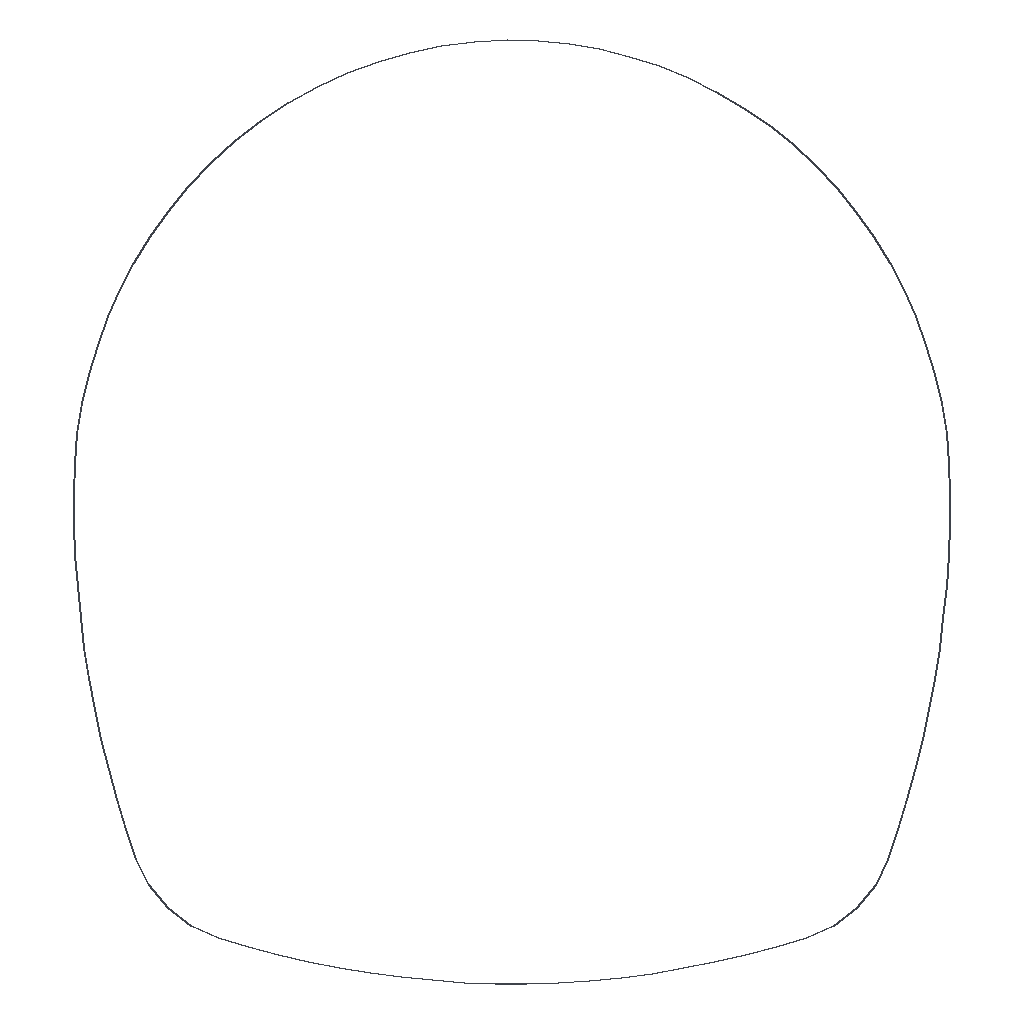Simulation study | abaqus
Set-up summary:
category,name,step,type,value,unit,region
solver,abaqus,,Abaqus/CAE 2024
units,SI m-kg-s (Pa),,inferred,E=3.25e+10 density=2500
analysis,Step-1,,static,time_period=1
mesh,nodes,,,96
mesh,elements,,,96
element_type,B21,,,96
material,Material-1,,E,3.25e+10
material,Material-1,,nu,0.2
material,Material-1,,density,2500
section,Material-1,,beam section,,,_PickedSet11
load,Load-1,Step-1,py,-430000,,_PickedSet9
load,Load-2,Step-1,py,660000,,_PickedSet10
load,Load-3,Step-1,px,-681730,,Part-1-1.37
load,Load-3,Step-1,px,-683457,,Part-1-1.38
load,Load-3,Step-1,px,-684985,,Part-1-1.39
load,Load-3,Step-1,px,-686311,,Part-1-1.40
load,Load-3,Step-1,px,-687434,,Part-1-1.41
load,Load-3,Step-1,px,-688353,,Part-1-1.42
load,Load-3,Step-1,px,-689067,,Part-1-1.43
load,Load-3,Step-1,px,-689576,,Part-1-1.44
load,Load-3,Step-1,px,-689878,,Part-1-1.45
load,Load-3,Step-1,px,-667487,,Part-1-1.46
load,Load-3,Step-1,px,-672461,,Part-1-1.47
load,Load-3,Step-1,px,-676572,,Part-1-1.48
load,Load-3,Step-1,px,-679599,,Part-1-1.49
load,Load-3,Step-1,px,-594403,,Part-1-1.50
load,Load-3,Step-1,px,-600644,,Part-1-1.51
load,Load-3,Step-1,px,-606879,,Part-1-1.52
load,Load-3,Step-1,px,-613101,,Part-1-1.53
load,Load-3,Step-1,px,-619306,,Part-1-1.54
load,Load-3,Step-1,px,-625489,,Part-1-1.55
load,Load-3,Step-1,px,-631645,,Part-1-1.56
load,Load-3,Step-1,px,-637769,,Part-1-1.57
load,Load-3,Step-1,px,-643857,,Part-1-1.58
load,Load-3,Step-1,px,-649903,,Part-1-1.59
load,Load-3,Step-1,px,-655904,,Part-1-1.60
load,Load-3,Step-1,px,-661854,,Part-1-1.61
load,Load-3,Step-1,px,-537041,,Part-1-1.62
load,Load-3,Step-1,px,-542130,,Part-1-1.63
load,Load-3,Step-1,px,-547422,,Part-1-1.64
load,Load-3,Step-1,px,-552895,,Part-1-1.65
load,Load-3,Step-1,px,-558528,,Part-1-1.66
load,Load-3,Step-1,px,-564296,,Part-1-1.67
load,Load-3,Step-1,px,-570176,,Part-1-1.68
load,Load-3,Step-1,px,-576143,,Part-1-1.69
load,Load-3,Step-1,px,-582173,,Part-1-1.70
load,Load-3,Step-1,px,-588240,,Part-1-1.71
load,Load-3,Step-1,px,-500019,,Part-1-1.72
load,Load-3,Step-1,px,-500401,,Part-1-1.73
load,Load-3,Step-1,px,-501231,,Part-1-1.74
load,Load-3,Step-1,px,-502505,,Part-1-1.75
load,Load-3,Step-1,px,-504216,,Part-1-1.76
load,Load-3,Step-1,px,-506356,,Part-1-1.77
load,Load-3,Step-1,px,-508912,,Part-1-1.78
load,Load-3,Step-1,px,-511872,,Part-1-1.79
load,Load-3,Step-1,px,-515221,,Part-1-1.80
load,Load-3,Step-1,px,-518940,,Part-1-1.81
load,Load-3,Step-1,px,-523011,,Part-1-1.82
load,Load-3,Step-1,px,-527413,,Part-1-1.83
load,Load-3,Step-1,px,-532122,,Part-1-1.84
load,Load-3-Copy,Step-1,px,588238,,Part-1-1.1
load,Load-3-Copy,Step-1,px,582171,,Part-1-1.2
load,Load-3-Copy,Step-1,px,576142,,Part-1-1.3
load,Load-3-Copy,Step-1,px,570175,,Part-1-1.4
load,Load-3-Copy,Step-1,px,564296,,Part-1-1.5
load,Load-3-Copy,Step-1,px,558528,,Part-1-1.6
load,Load-3-Copy,Step-1,px,552896,,Part-1-1.7
load,Load-3-Copy,Step-1,px,547422,,Part-1-1.8
load,Load-3-Copy,Step-1,px,542130,,Part-1-1.9
load,Load-3-Copy,Step-1,px,537041,,Part-1-1.10
load,Load-3-Copy,Step-1,px,661837,,Part-1-1.11
load,Load-3-Copy,Step-1,px,655888,,Part-1-1.12
load,Load-3-Copy,Step-1,px,649888,,Part-1-1.13
load,Load-3-Copy,Step-1,px,643842,,Part-1-1.14
load,Load-3-Copy,Step-1,px,637755,,Part-1-1.15
load,Load-3-Copy,Step-1,px,631632,,Part-1-1.16
load,Load-3-Copy,Step-1,px,625477,,Part-1-1.17
load,Load-3-Copy,Step-1,px,619296,,Part-1-1.18
load,Load-3-Copy,Step-1,px,613093,,Part-1-1.19
load,Load-3-Copy,Step-1,px,606872,,Part-1-1.20
load,Load-3-Copy,Step-1,px,600640,,Part-1-1.21
load,Load-3-Copy,Step-1,px,594400,,Part-1-1.22
load,Load-3-Copy,Step-1,px,679583,,Part-1-1.23
load,Load-3-Copy,Step-1,px,676500,,Part-1-1.24
load,Load-3-Copy,Step-1,px,672388,,Part-1-1.25
load,Load-3-Copy,Step-1,px,667448,,Part-1-1.26
load,Load-3-Copy,Step-1,px,689975,,Part-1-1.27
load,Load-3-Copy,Step-1,px,689866,,Part-1-1.28
load,Load-3-Copy,Step-1,px,689555,,Part-1-1.29
load,Load-3-Copy,Step-1,px,689042,,Part-1-1.30
load,Load-3-Copy,Step-1,px,688326,,Part-1-1.31
load,Load-3-Copy,Step-1,px,687409,,Part-1-1.32
load,Load-3-Copy,Step-1,px,686292,,Part-1-1.33
load,Load-3-Copy,Step-1,px,684975,,Part-1-1.34
load,Load-3-Copy,Step-1,px,683461,,Part-1-1.35
load,Load-3-Copy,Step-1,px,681750,,Part-1-1.36
load,Load-3-Copy,Step-1,px,531985,,Part-1-1.85
load,Load-3-Copy,Step-1,px,527021,,Part-1-1.86
load,Load-3-Copy,Step-1,px,522403,,Part-1-1.87
load,Load-3-Copy,Step-1,px,518159,,Part-1-1.88
load,Load-3-Copy,Step-1,px,514313,,Part-1-1.89
load,Load-3-Copy,Step-1,px,510888,,Part-1-1.90
load,Load-3-Copy,Step-1,px,507903,,Part-1-1.91
load,Load-3-Copy,Step-1,px,505377,,Part-1-1.92
load,Load-3-Copy,Step-1,px,503323,,Part-1-1.93
load,Load-3-Copy,Step-1,px,501753,,Part-1-1.94
load,Load-3-Copy,Step-1,px,500678,,Part-1-1.95
load,Load-3-Copy,Step-1,px,500102,,Part-1-1.96
bc,BC-1,Step-1,fixed,[dofs=y],,_PickedSet13
Abaqus input file, long lists of numbers shortened:
*Heading
** Job name: deck Model name: Model-1
** Generated by: Abaqus/CAE 2024
*Preprint, echo=NO, model=NO, history=NO, contact=NO
**
** PARTS
**
*Part, name=Part-1
*Node
      1,   1.803,    6.083
      2,   1.213,    4.313
** (94 more lines like these left out)
*Element, type=B21
 1,  2, 11
 2, 11, 12
** (94 more lines like these left out)
*Nset, nset=_PickedSet11, internal, generate
  1,  96,   1
*Elset, elset=_PickedSet11, internal, generate
  1,  96,   1
** Section: Section-2  Profile: Profile-1
*Beam Section, elset=_PickedSet11, material=Material-1, temperature=GRADIENTS, section=RECT
0.4, 1.
0.,0.,-1.
*End Part
**
**
** ASSEMBLY
**
*Assembly, name=Assembly
**
*Instance, name=Part-1-1, part=Part-1
   -3.965,    -1.233,           0.
*End Instance
**
*Nset, nset=_PickedSet9, internal, instance=Part-1-1
  1,  2,  8,  9, 10, 11, 12, 13, 14, 15, 16, 17, 18, 19, 65, 66
 67, 68, 69, 70, 71, 72, 73, 74, 75, 76, 77, 78, 79, 80, 81, 82
** (1 more lines like these left out)
*Elset, elset=_PickedSet9, internal, instance=Part-1-1
  1,  2,  3,  4,  5,  6,  7,  8,  9, 10, 62, 63, 64, 65, 66, 67
 68, 69, 70, 71, 72, 73, 74, 75, 76, 77, 78, 79, 80, 81, 82, 83
** (1 more lines like these left out)
*Nset, nset=_PickedSet10, internal, instance=Part-1-1
  2,  3,  4,  5,  6,  7,  8, 20, 21, 22, 23, 24, 25, 26, 27, 28
 29, 30, 31, 32, 33, 34, 35, 36, 37, 38, 39, 40, 41, 42, 43, 44
** (2 more lines like these left out)
*Elset, elset=_PickedSet10, internal, instance=Part-1-1, generate
 11,  61,   1
*Nset, nset=_PickedSet11, internal, instance=Part-1-1
  5,  6,  7,  8,  9, 10, 43, 44, 45, 46, 47, 48, 49, 50, 51, 52
 53, 54, 55, 56, 57, 58, 59, 60, 61, 62, 63, 64, 65, 66, 67, 68
** (2 more lines like these left out)
*Elset, elset=_PickedSet11, internal, instance=Part-1-1, generate
 37,  84,   1
*Nset, nset=_PickedSet12, internal, instance=Part-1-1
  1,  2,  3,  4,  5, 10, 11, 12, 13, 14, 15, 16, 17, 18, 19, 20
 21, 22, 23, 24, 25, 26, 27, 28, 29, 30, 31, 32, 33, 34, 35, 36
** (2 more lines like these left out)
*Elset, elset=_PickedSet12, internal, instance=Part-1-1
  1,  2,  3,  4,  5,  6,  7,  8,  9, 10, 11, 12, 13, 14, 15, 16
 17, 18, 19, 20, 21, 22, 23, 24, 25, 26, 27, 28, 29, 30, 31, 32
** (1 more lines like these left out)
*Nset, nset=_PickedSet13, internal, instance=Part-1-1
 4, 6
*End Assembly
**
** MATERIALS
**
*Material, name=Material-1
*Density
2500.,
*Elastic
 3.25e+10, 0.2
** ----------------------------------------------------------------
**
** STEP: Step-1
**
*Step, name=Step-1, nlgeom=NO, inc=100000
*Static, stabilize=0.0002, allsdtol=0.05, continue=NO
0.1, 1., 1e-08, 1.
**
** BOUNDARY CONDITIONS
**
** Name: BC-1 Type: Displacement/Rotation
*Boundary
_PickedSet13, 2, 2
**
** LOADS
**
** Name: Load-1   Type: Line load
*Dload, op=NEW
_PickedSet9, PY, -430000.
** Name: Load-2   Type: Line load
*Dload, op=NEW
_PickedSet10, PY, 660000.
** Name: Load-3   Type: Line load Using Field: AnalyticalField-1
*Dload, op=NEW
Part-1-1.37, PX, -681730.
Part-1-1.38, PX, -683457.
Part-1-1.39, PX, -684985.
Part-1-1.40, PX, -686311.
Part-1-1.41, PX, -687434.
Part-1-1.42, PX, -688353.
Part-1-1.43, PX, -689067.
Part-1-1.44, PX, -689576.
Part-1-1.45, PX, -689878.
Part-1-1.46, PX, -667487.
Part-1-1.47, PX, -672461.
Part-1-1.48, PX, -676572.
Part-1-1.49, PX, -679599.
Part-1-1.50, PX, -594403.
Part-1-1.51, PX, -600644.
Part-1-1.52, PX, -606879.
Part-1-1.53, PX, -613101.
Part-1-1.54, PX, -619306.
Part-1-1.55, PX, -625489.
Part-1-1.56, PX, -631645.
Part-1-1.57, PX, -637769.
Part-1-1.58, PX, -643857.
Part-1-1.59, PX, -649903.
Part-1-1.60, PX, -655904.
Part-1-1.61, PX, -661854.
Part-1-1.62, PX, -537041.
Part-1-1.63, PX, -542130.
Part-1-1.64, PX, -547422.
Part-1-1.65, PX, -552895.
Part-1-1.66, PX, -558528.
Part-1-1.67, PX, -564296.
Part-1-1.68, PX, -570176.
Part-1-1.69, PX, -576143.
Part-1-1.70, PX, -582173.
Part-1-1.71, PX, -588240.
Part-1-1.72, PX, -500019.
Part-1-1.73, PX, -500401.
Part-1-1.74, PX, -501231.
Part-1-1.75, PX, -502505.
Part-1-1.76, PX, -504216.
** (8 more lines like these left out)
** Name: Load-3-Copy   Type: Line load Using Field: AnalyticalField-1
*Dload, op=NEW
Part-1-1.1, PX, 588238.
Part-1-1.2, PX, 582171.
Part-1-1.3, PX, 576142.
Part-1-1.4, PX, 570175.
Part-1-1.5, PX, 564296.
Part-1-1.6, PX, 558528.
Part-1-1.7, PX, 552896.
Part-1-1.8, PX, 547422.
Part-1-1.9, PX, 542130.
Part-1-1.10, PX, 537041.
Part-1-1.11, PX, 661837.
Part-1-1.12, PX, 655888.
Part-1-1.13, PX, 649888.
Part-1-1.14, PX, 643842.
Part-1-1.15, PX, 637755.
Part-1-1.16, PX, 631632.
Part-1-1.17, PX, 625477.
Part-1-1.18, PX, 619296.
Part-1-1.19, PX, 613093.
Part-1-1.20, PX, 606872.
Part-1-1.21, PX, 600640.
Part-1-1.22, PX, 594400.
Part-1-1.23, PX, 679583.
Part-1-1.24, PX, 676500.
Part-1-1.25, PX, 672388.
Part-1-1.26, PX, 667448.
Part-1-1.27, PX, 689975.
Part-1-1.28, PX, 689866.
Part-1-1.29, PX, 689555.
Part-1-1.30, PX, 689042.
Part-1-1.31, PX, 688326.
Part-1-1.32, PX, 687409.
Part-1-1.33, PX, 686292.
Part-1-1.34, PX, 684975.
Part-1-1.35, PX, 683461.
Part-1-1.36, PX, 681750.
Part-1-1.85, PX, 531985.
Part-1-1.86, PX, 527021.
Part-1-1.87, PX, 522403.
Part-1-1.88, PX, 518159.
** (8 more lines like these left out)
**
** OUTPUT REQUESTS
**
*Restart, write, frequency=0
**
** FIELD OUTPUT: F-Output-1
**
*Output, field
*Node Output
CF, RF, U
*Element Output, directions=YES
LE, PE, PEEQ, PEMAG, S, SF
*Contact Output
CDISP, CSTRESS
**
** HISTORY OUTPUT: H-Output-1
**
*Output, history, variable=PRESELECT
*End Step
Results summary:
result,odb.job_status,,,JOB_STATUS_COMPLETED_SUCCESSFULLY,"consistent, unstated (Abaqus has no unit system)"
result,steps[0].procedure,Step-1,,*STATIC,"consistent, unstated (Abaqus has no unit system)"
result,steps[0].time_period,Step-1,,1,"consistent, unstated (Abaqus has no unit system)"
result,steps[0].n_frames,Step-1,,10,"consistent, unstated (Abaqus has no unit system)"
result,steps[0].last_frame.id,Step-1,,9,"consistent, unstated (Abaqus has no unit system)"
result,steps[0].last_frame.value,Step-1,,1,"consistent, unstated (Abaqus has no unit system)"
result,steps[0].last_frame.description,Step-1,,Increment      9: Step Time =    1.000,"consistent, unstated (Abaqus has no unit system)"
result,steps[0].completed,Step-1,,True,"consistent, unstated (Abaqus has no unit system)"
result,steps[0].max_U_magnitude,Step-1,,26.21,"consistent, unstated (Abaqus has no unit system)"
result,steps[0].max_S_mises,Step-1,,1.77461e+07,"consistent, unstated (Abaqus has no unit system)"
result,steps[0].RF_sum[1],Step-1,,0,"consistent, unstated (Abaqus has no unit system)"
result,steps[0].RF_sum[2],Step-1,,-2.7549e+06,"consistent, unstated (Abaqus has no unit system)"